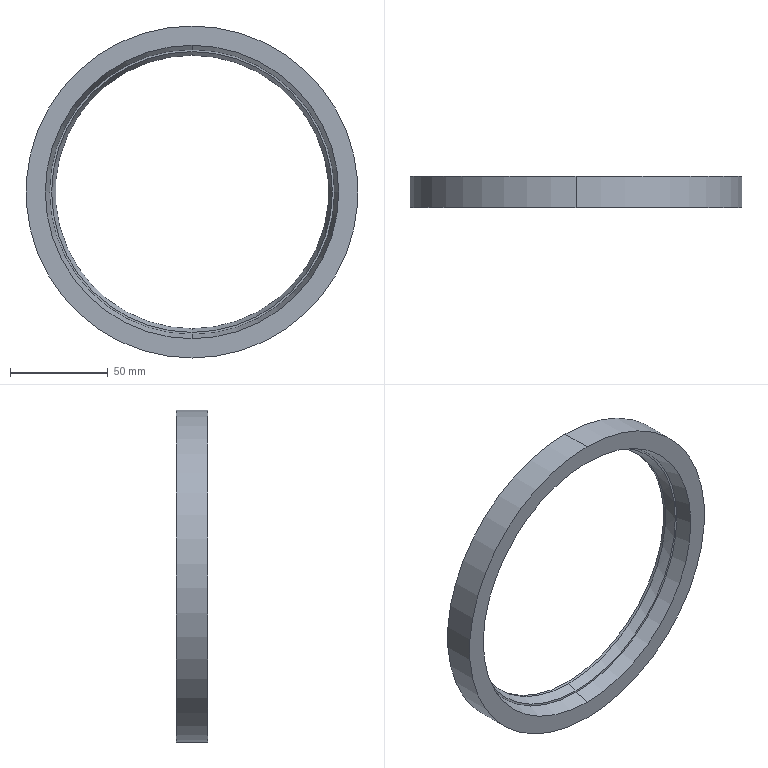Part | STEP file | JB1091-1991 skeleton-type vacuum rubber seal ring 140 | 1 solid | 23 faces | box 170 x 16 x 170 mm | volume 62160 mm3 | cone 8 | cylinder 6 | plane 5 | torus 4 | commonest cylinder face diameters 140 x2 152.823 x2 170 x2
STEP:
#1=CARTESIAN_POINT('',(0.,0.,0.));
#2=DIRECTION('',(0.,0.,1.));
#3=DIRECTION('',(1.,0.,0.));
#4=AXIS2_PLACEMENT_3D('',#1,#2,#3);
#5=CARTESIAN_POINT('',(0.,13.014,76.412));
#6=VERTEX_POINT('',#5);
#7=CARTESIAN_POINT('',(0.,13.014,-76.412));
#8=VERTEX_POINT('',#7);
#9=CARTESIAN_POINT('',(0.,13.014,0.));
#10=DIRECTION('',(0.,1.,0.));
#11=DIRECTION('',(0.,0.,1.));
#12=AXIS2_PLACEMENT_3D('',#9,#10,#11);
#13=CIRCLE('',#12,76.412);
#14=CARTESIAN_POINT('',(0.,10.581,0.));
#15=DIRECTION('',(0.,1.,0.));
#16=DIRECTION('',(0.,0.,1.));
#17=AXIS2_PLACEMENT_3D('',#14,#15,#16);
#18=TOROIDAL_SURFACE('',#17,75.552,2.581);
#19=CARTESIAN_POINT('',(0.,1.231));
#20=DIRECTION('',(1.,0.));
#21=VECTOR('',#20,1.);
#22=LINE('',#19,#21);
#23=(GEOMETRIC_REPRESENTATION_CONTEXT(2)PARAMETRIC_REPRESENTATION_CONTEXT()REPRESENTATION_CONTEXT('',''));
#24=DEFINITIONAL_REPRESENTATION('',(#22),#23);
#25=PCURVE('',#18,#24);
#26=CARTESIAN_POINT('',(0.,0.,0.));
#27=DIRECTION('',(0.,1.,0.));
#28=DIRECTION('',(0.,0.,1.));
#29=AXIS2_PLACEMENT_3D('',#26,#27,#28);
#30=CYLINDRICAL_SURFACE('',#29,76.412);
#31=CARTESIAN_POINT('',(0.,13.014));
#32=DIRECTION('',(1.,0.));
#33=VECTOR('',#32,1.);
#34=LINE('',#31,#33);
#35=(GEOMETRIC_REPRESENTATION_CONTEXT(2)PARAMETRIC_REPRESENTATION_CONTEXT()REPRESENTATION_CONTEXT('',''));
#36=DEFINITIONAL_REPRESENTATION('',(#34),#35);
#37=PCURVE('',#30,#36);
#38=SURFACE_CURVE('',#13,(#25,#37),.PCURVE_S1.);
#39=EDGE_CURVE('',#6,#8,#38,.T.);
#40=ORIENTED_EDGE('',*,*,#39,.T.);
#41=CARTESIAN_POINT('',(0.,10.581,-72.971));
#42=VERTEX_POINT('',#41);
#43=CARTESIAN_POINT('',(0.,10.581,-75.552));
#44=DIRECTION('',(1.,0.,0.));
#45=DIRECTION('',(0.,0.,-1.));
#46=AXIS2_PLACEMENT_3D('',#43,#44,#45);
#47=CIRCLE('',#46,2.581);
#48=CARTESIAN_POINT('',(3.142,0.));
#49=DIRECTION('',(0.,1.));
#50=VECTOR('',#49,1.);
#51=LINE('',#48,#50);
#52=(GEOMETRIC_REPRESENTATION_CONTEXT(2)PARAMETRIC_REPRESENTATION_CONTEXT()REPRESENTATION_CONTEXT('',''));
#53=DEFINITIONAL_REPRESENTATION('',(#51),#52);
#54=PCURVE('',#18,#53);
#55=CARTESIAN_POINT('',(0.,10.581,0.));
#56=DIRECTION('',(0.,1.,0.));
#57=DIRECTION('',(0.,0.,1.));
#58=AXIS2_PLACEMENT_3D('',#55,#56,#57);
#59=TOROIDAL_SURFACE('',#58,75.552,2.581);
#60=CARTESIAN_POINT('',(3.142,0.));
#61=DIRECTION('',(0.,1.));
#62=VECTOR('',#61,1.);
#63=LINE('',#60,#62);
#64=(GEOMETRIC_REPRESENTATION_CONTEXT(2)PARAMETRIC_REPRESENTATION_CONTEXT()REPRESENTATION_CONTEXT('',''));
#65=DEFINITIONAL_REPRESENTATION('',(#63),#64);
#66=PCURVE('',#59,#65);
#67=SURFACE_CURVE('',#47,(#54,#66),.PCURVE_S1.);
#68=EDGE_CURVE('',#8,#42,#67,.T.);
#69=ORIENTED_EDGE('',*,*,#68,.T.);
#70=CARTESIAN_POINT('',(0.,10.581,72.971));
#71=VERTEX_POINT('',#70);
#72=CARTESIAN_POINT('',(0.,10.581,0.));
#73=DIRECTION('',(0.,1.,0.));
#74=DIRECTION('',(0.,0.,1.));
#75=AXIS2_PLACEMENT_3D('',#72,#73,#74);
#76=CIRCLE('',#75,72.971);
#77=CARTESIAN_POINT('',(0.,3.142));
#78=DIRECTION('',(1.,0.));
#79=VECTOR('',#78,1.);
#80=LINE('',#77,#79);
#81=(GEOMETRIC_REPRESENTATION_CONTEXT(2)PARAMETRIC_REPRESENTATION_CONTEXT()REPRESENTATION_CONTEXT('',''));
#82=DEFINITIONAL_REPRESENTATION('',(#80),#81);
#83=PCURVE('',#18,#82);
#84=CARTESIAN_POINT('',(0.,10.581,0.));
#85=DIRECTION('',(0.,1.,0.));
#86=DIRECTION('',(0.,0.,1.));
#87=AXIS2_PLACEMENT_3D('',#84,#85,#86);
#88=TOROIDAL_SURFACE('',#87,75.552,2.581);
#89=CARTESIAN_POINT('',(0.,3.142));
#90=DIRECTION('',(1.,0.));
#91=VECTOR('',#90,1.);
#92=LINE('',#89,#91);
#93=(GEOMETRIC_REPRESENTATION_CONTEXT(2)PARAMETRIC_REPRESENTATION_CONTEXT()REPRESENTATION_CONTEXT('',''));
#94=DEFINITIONAL_REPRESENTATION('',(#92),#93);
#95=PCURVE('',#88,#94);
#96=SURFACE_CURVE('',#76,(#83,#95),.PCURVE_S1.);
#97=EDGE_CURVE('',#71,#42,#96,.T.);
#98=ORIENTED_EDGE('',*,*,#97,.F.);
#99=CARTESIAN_POINT('',(0.,10.581,75.552));
#100=DIRECTION('',(-1.,0.,0.));
#101=DIRECTION('',(0.,0.,1.));
#102=AXIS2_PLACEMENT_3D('',#99,#100,#101);
#103=CIRCLE('',#102,2.581);
#104=CARTESIAN_POINT('',(0.,0.));
#105=DIRECTION('',(0.,1.));
#106=VECTOR('',#105,1.);
#107=LINE('',#104,#106);
#108=(GEOMETRIC_REPRESENTATION_CONTEXT(2)PARAMETRIC_REPRESENTATION_CONTEXT()REPRESENTATION_CONTEXT('',''));
#109=DEFINITIONAL_REPRESENTATION('',(#107),#108);
#110=PCURVE('',#18,#109);
#111=CARTESIAN_POINT('',(6.283,0.));
#112=DIRECTION('',(0.,1.));
#113=VECTOR('',#112,1.);
#114=LINE('',#111,#113);
#115=(GEOMETRIC_REPRESENTATION_CONTEXT(2)PARAMETRIC_REPRESENTATION_CONTEXT()REPRESENTATION_CONTEXT('',''));
#116=DEFINITIONAL_REPRESENTATION('',(#114),#115);
#117=PCURVE('',#59,#116);
#118=SURFACE_CURVE('',#103,(#110,#117),.PCURVE_S1.);
#119=EDGE_CURVE('',#6,#71,#118,.T.);
#120=ORIENTED_EDGE('',*,*,#119,.F.);
#121=EDGE_LOOP('',(#40,#69,#98,#120));
#122=FACE_BOUND('',#121,.F.);
#123=ADVANCED_FACE('',(#122),#18,.F.);
#124=CARTESIAN_POINT('',(0.,13.014,0.));
#125=DIRECTION('',(0.,1.,0.));
#126=DIRECTION('',(0.,0.,1.));
#127=AXIS2_PLACEMENT_3D('',#124,#125,#126);
#128=CIRCLE('',#127,76.412);
#129=CARTESIAN_POINT('',(0.,1.231));
#130=DIRECTION('',(1.,0.));
#131=VECTOR('',#130,1.);
#132=LINE('',#129,#131);
#133=(GEOMETRIC_REPRESENTATION_CONTEXT(2)PARAMETRIC_REPRESENTATION_CONTEXT()REPRESENTATION_CONTEXT('',''));
#134=DEFINITIONAL_REPRESENTATION('',(#132),#133);
#135=PCURVE('',#59,#134);
#136=CARTESIAN_POINT('',(0.,0.,0.));
#137=DIRECTION('',(0.,1.,0.));
#138=DIRECTION('',(0.,0.,1.));
#139=AXIS2_PLACEMENT_3D('',#136,#137,#138);
#140=CYLINDRICAL_SURFACE('',#139,76.412);
#141=CARTESIAN_POINT('',(0.,13.014));
#142=DIRECTION('',(1.,0.));
#143=VECTOR('',#142,1.);
#144=LINE('',#141,#143);
#145=(GEOMETRIC_REPRESENTATION_CONTEXT(2)PARAMETRIC_REPRESENTATION_CONTEXT()REPRESENTATION_CONTEXT('',''));
#146=DEFINITIONAL_REPRESENTATION('',(#144),#145);
#147=PCURVE('',#140,#146);
#148=SURFACE_CURVE('',#128,(#135,#147),.PCURVE_S1.);
#149=EDGE_CURVE('',#8,#6,#148,.T.);
#150=ORIENTED_EDGE('',*,*,#149,.T.);
#151=ORIENTED_EDGE('',*,*,#119,.T.);
#152=CARTESIAN_POINT('',(0.,10.581,0.));
#153=DIRECTION('',(0.,1.,0.));
#154=DIRECTION('',(0.,0.,1.));
#155=AXIS2_PLACEMENT_3D('',#152,#153,#154);
#156=CIRCLE('',#155,72.971);
#157=CARTESIAN_POINT('',(0.,3.142));
#158=DIRECTION('',(1.,0.));
#159=VECTOR('',#158,1.);
#160=LINE('',#157,#159);
#161=(GEOMETRIC_REPRESENTATION_CONTEXT(2)PARAMETRIC_REPRESENTATION_CONTEXT()REPRESENTATION_CONTEXT('',''));
#162=DEFINITIONAL_REPRESENTATION('',(#160),#161);
#163=PCURVE('',#59,#162);
#164=CARTESIAN_POINT('',(0.,10.581,0.));
#165=DIRECTION('',(0.,1.,0.));
#166=DIRECTION('',(0.,0.,1.));
#167=AXIS2_PLACEMENT_3D('',#164,#165,#166);
#168=TOROIDAL_SURFACE('',#167,75.552,2.581);
#169=CARTESIAN_POINT('',(0.,3.142));
#170=DIRECTION('',(1.,0.));
#171=VECTOR('',#170,1.);
#172=LINE('',#169,#171);
#173=(GEOMETRIC_REPRESENTATION_CONTEXT(2)PARAMETRIC_REPRESENTATION_CONTEXT()REPRESENTATION_CONTEXT('',''));
#174=DEFINITIONAL_REPRESENTATION('',(#172),#173);
#175=PCURVE('',#168,#174);
#176=SURFACE_CURVE('',#156,(#163,#175),.PCURVE_S1.);
#177=EDGE_CURVE('',#42,#71,#176,.T.);
#178=ORIENTED_EDGE('',*,*,#177,.F.);
#179=ORIENTED_EDGE('',*,*,#68,.F.);
#180=EDGE_LOOP('',(#150,#151,#178,#179));
#181=FACE_BOUND('',#180,.F.);
#182=ADVANCED_FACE('',(#181),#59,.F.);
#183=CARTESIAN_POINT('',(0.,0.,85.));
#184=VERTEX_POINT('',#183);
#185=CARTESIAN_POINT('',(0.,0.,-85.));
#186=VERTEX_POINT('',#185);
#187=CARTESIAN_POINT('',(0.,0.,0.));
#188=DIRECTION('',(0.,1.,0.));
#189=DIRECTION('',(0.,0.,1.));
#190=AXIS2_PLACEMENT_3D('',#187,#188,#189);
#191=CIRCLE('',#190,85.);
#192=CARTESIAN_POINT('',(0.,0.,0.));
#193=DIRECTION('',(0.,1.,0.));
#194=DIRECTION('',(0.,0.,1.));
#195=AXIS2_PLACEMENT_3D('',#192,#193,#194);
#196=CYLINDRICAL_SURFACE('',#195,85.);
#197=CARTESIAN_POINT('',(0.,0.));
#198=DIRECTION('',(1.,0.));
#199=VECTOR('',#198,1.);
#200=LINE('',#197,#199);
#201=(GEOMETRIC_REPRESENTATION_CONTEXT(2)PARAMETRIC_REPRESENTATION_CONTEXT()REPRESENTATION_CONTEXT('',''));
#202=DEFINITIONAL_REPRESENTATION('',(#200),#201);
#203=PCURVE('',#196,#202);
#204=CARTESIAN_POINT('',(-85.,0.,0.));
#205=DIRECTION('',(0.,-1.,0.));
#206=DIRECTION('',(0.,0.,-1.));
#207=AXIS2_PLACEMENT_3D('',#204,#205,#206);
#208=PLANE('',#207);
#209=CARTESIAN_POINT('',(-85.,85.));
#210=CARTESIAN_POINT('',(-85.,232.224));
#211=CARTESIAN_POINT('',(42.5,158.612));
#212=CARTESIAN_POINT('',(170.,85.));
#213=CARTESIAN_POINT('',(42.5,11.388));
#214=CARTESIAN_POINT('',(-85.,-62.224));
#215=CARTESIAN_POINT('',(-85.,85.));
#216=(BOUNDED_CURVE()B_SPLINE_CURVE(2,(#209,#210,#211,#212,#213,#214,#215),.UNSPECIFIED.,.T.,.F.)B_SPLINE_CURVE_WITH_KNOTS((1,2,2,2,2,1),(-2.094,0.,2.094,4.189,6.283,8.378),.UNSPECIFIED.)CURVE()GEOMETRIC_REPRESENTATION_ITEM()RATIONAL_B_SPLINE_CURVE((1.,0.5,1.,0.5,1.,0.5,1.))REPRESENTATION_ITEM(''));
#217=(GEOMETRIC_REPRESENTATION_CONTEXT(2)PARAMETRIC_REPRESENTATION_CONTEXT()REPRESENTATION_CONTEXT('',''));
#218=DEFINITIONAL_REPRESENTATION('',(#216),#217);
#219=PCURVE('',#208,#218);
#220=SURFACE_CURVE('',#191,(#203,#219),.PCURVE_S1.);
#221=EDGE_CURVE('',#184,#186,#220,.T.);
#222=ORIENTED_EDGE('',*,*,#221,.T.);
#223=CARTESIAN_POINT('',(0.,16.,-85.));
#224=VERTEX_POINT('',#223);
#225=CARTESIAN_POINT('',(0.,0.,-85.));
#226=DIRECTION('',(0.,1.,0.));
#227=VECTOR('',#226,1.);
#228=LINE('',#225,#227);
#229=CARTESIAN_POINT('',(3.142,0.));
#230=DIRECTION('',(0.,1.));
#231=VECTOR('',#230,1.);
#232=LINE('',#229,#231);
#233=(GEOMETRIC_REPRESENTATION_CONTEXT(2)PARAMETRIC_REPRESENTATION_CONTEXT()REPRESENTATION_CONTEXT('',''));
#234=DEFINITIONAL_REPRESENTATION('',(#232),#233);
#235=PCURVE('',#196,#234);
#236=CARTESIAN_POINT('',(0.,0.,0.));
#237=DIRECTION('',(0.,1.,0.));
#238=DIRECTION('',(0.,0.,1.));
#239=AXIS2_PLACEMENT_3D('',#236,#237,#238);
#240=CYLINDRICAL_SURFACE('',#239,85.);
#241=CARTESIAN_POINT('',(3.142,0.));
#242=DIRECTION('',(0.,1.));
#243=VECTOR('',#242,1.);
#244=LINE('',#241,#243);
#245=(GEOMETRIC_REPRESENTATION_CONTEXT(2)PARAMETRIC_REPRESENTATION_CONTEXT()REPRESENTATION_CONTEXT('',''));
#246=DEFINITIONAL_REPRESENTATION('',(#244),#245);
#247=PCURVE('',#240,#246);
#248=SURFACE_CURVE('',#228,(#235,#247),.PCURVE_S1.);
#249=EDGE_CURVE('',#186,#224,#248,.T.);
#250=ORIENTED_EDGE('',*,*,#249,.T.);
#251=CARTESIAN_POINT('',(0.,16.,85.));
#252=VERTEX_POINT('',#251);
#253=CARTESIAN_POINT('',(0.,16.,0.));
#254=DIRECTION('',(0.,1.,0.));
#255=DIRECTION('',(0.,0.,1.));
#256=AXIS2_PLACEMENT_3D('',#253,#254,#255);
#257=CIRCLE('',#256,85.);
#258=CARTESIAN_POINT('',(0.,16.));
#259=DIRECTION('',(1.,0.));
#260=VECTOR('',#259,1.);
#261=LINE('',#258,#260);
#262=(GEOMETRIC_REPRESENTATION_CONTEXT(2)PARAMETRIC_REPRESENTATION_CONTEXT()REPRESENTATION_CONTEXT('',''));
#263=DEFINITIONAL_REPRESENTATION('',(#261),#262);
#264=PCURVE('',#196,#263);
#265=CARTESIAN_POINT('',(-82.419,16.,0.));
#266=DIRECTION('',(0.,1.,0.));
#267=DIRECTION('',(0.,0.,1.));
#268=AXIS2_PLACEMENT_3D('',#265,#266,#267);
#269=PLANE('',#268);
#270=CARTESIAN_POINT('',(0.,82.419));
#271=DIRECTION('',(1.,0.));
#272=AXIS2_PLACEMENT_2D('',#270,#271);
#273=CIRCLE('',#272,85.);
#274=(GEOMETRIC_REPRESENTATION_CONTEXT(2)PARAMETRIC_REPRESENTATION_CONTEXT()REPRESENTATION_CONTEXT('',''));
#275=DEFINITIONAL_REPRESENTATION('',(#273),#274);
#276=PCURVE('',#269,#275);
#277=SURFACE_CURVE('',#257,(#264,#276),.PCURVE_S1.);
#278=EDGE_CURVE('',#252,#224,#277,.T.);
#279=ORIENTED_EDGE('',*,*,#278,.F.);
#280=CARTESIAN_POINT('',(0.,0.,85.));
#281=DIRECTION('',(0.,1.,0.));
#282=VECTOR('',#281,1.);
#283=LINE('',#280,#282);
#284=CARTESIAN_POINT('',(0.,0.));
#285=DIRECTION('',(0.,1.));
#286=VECTOR('',#285,1.);
#287=LINE('',#284,#286);
#288=(GEOMETRIC_REPRESENTATION_CONTEXT(2)PARAMETRIC_REPRESENTATION_CONTEXT()REPRESENTATION_CONTEXT('',''));
#289=DEFINITIONAL_REPRESENTATION('',(#287),#288);
#290=PCURVE('',#196,#289);
#291=CARTESIAN_POINT('',(6.283,0.));
#292=DIRECTION('',(0.,1.));
#293=VECTOR('',#292,1.);
#294=LINE('',#291,#293);
#295=(GEOMETRIC_REPRESENTATION_CONTEXT(2)PARAMETRIC_REPRESENTATION_CONTEXT()REPRESENTATION_CONTEXT('',''));
#296=DEFINITIONAL_REPRESENTATION('',(#294),#295);
#297=PCURVE('',#240,#296);
#298=SURFACE_CURVE('',#283,(#290,#297),.PCURVE_S1.);
#299=EDGE_CURVE('',#184,#252,#298,.T.);
#300=ORIENTED_EDGE('',*,*,#299,.F.);
#301=EDGE_LOOP('',(#222,#250,#279,#300));
#302=FACE_BOUND('',#301,.T.);
#303=ADVANCED_FACE('',(#302),#196,.T.);
#304=CARTESIAN_POINT('',(0.,8.,-72.971));
#305=VERTEX_POINT('',#304);
#306=CARTESIAN_POINT('',(0.,0.,-75.114));
#307=VERTEX_POINT('',#306);
#308=CARTESIAN_POINT('',(0.,0.,-75.114));
#309=DIRECTION('',(0.,-0.9659,-0.2588));
#310=VECTOR('',#309,1.);
#311=LINE('',#308,#310);
#312=CARTESIAN_POINT('',(0.,0.,0.));
#313=DIRECTION('',(0.,-1.,0.));
#314=DIRECTION('',(0.,0.,-1.));
#315=AXIS2_PLACEMENT_3D('',#312,#313,#314);
#316=CONICAL_SURFACE('',#315,75.114,0.2618);
#317=CARTESIAN_POINT('',(6.283,0.));
#318=DIRECTION('',(0.,1.));
#319=VECTOR('',#318,1.);
#320=LINE('',#317,#319);
#321=(GEOMETRIC_REPRESENTATION_CONTEXT(2)PARAMETRIC_REPRESENTATION_CONTEXT()REPRESENTATION_CONTEXT('',''));
#322=DEFINITIONAL_REPRESENTATION('',(#320),#321);
#323=PCURVE('',#316,#322);
#324=CARTESIAN_POINT('',(0.,0.,0.));
#325=DIRECTION('',(0.,-1.,0.));
#326=DIRECTION('',(0.,0.,-1.));
#327=AXIS2_PLACEMENT_3D('',#324,#325,#326);
#328=CONICAL_SURFACE('',#327,75.114,0.2618);
#329=CARTESIAN_POINT('',(0.,0.));
#330=DIRECTION('',(0.,1.));
#331=VECTOR('',#330,1.);
#332=LINE('',#329,#331);
#333=(GEOMETRIC_REPRESENTATION_CONTEXT(2)PARAMETRIC_REPRESENTATION_CONTEXT()REPRESENTATION_CONTEXT('',''));
#334=DEFINITIONAL_REPRESENTATION('',(#332),#333);
#335=PCURVE('',#328,#334);
#336=SURFACE_CURVE('',#311,(#323,#335),.PCURVE_S1.);
#337=EDGE_CURVE('',#305,#307,#336,.T.);
#338=ORIENTED_EDGE('',*,*,#337,.T.);
#339=CARTESIAN_POINT('',(0.,0.,75.114));
#340=VERTEX_POINT('',#339);
#341=CARTESIAN_POINT('',(0.,0.,0.));
#342=DIRECTION('',(0.,1.,0.));
#343=DIRECTION('',(0.,0.,1.));
#344=AXIS2_PLACEMENT_3D('',#341,#342,#343);
#345=CIRCLE('',#344,75.114);
#346=CARTESIAN_POINT('',(9.425,0.));
#347=DIRECTION('',(-1.,0.));
#348=VECTOR('',#347,1.);
#349=LINE('',#346,#348);
#350=(GEOMETRIC_REPRESENTATION_CONTEXT(2)PARAMETRIC_REPRESENTATION_CONTEXT()REPRESENTATION_CONTEXT('',''));
#351=DEFINITIONAL_REPRESENTATION('',(#349),#350);
#352=PCURVE('',#316,#351);
#353=CARTESIAN_POINT('',(-75.114,85.));
#354=CARTESIAN_POINT('',(-75.114,215.102));
#355=CARTESIAN_POINT('',(37.557,150.051));
#356=CARTESIAN_POINT('',(150.229,85.));
#357=CARTESIAN_POINT('',(37.557,19.949));
#358=CARTESIAN_POINT('',(-75.114,-45.102));
#359=CARTESIAN_POINT('',(-75.114,85.));
#360=(BOUNDED_CURVE()B_SPLINE_CURVE(2,(#353,#354,#355,#356,#357,#358,#359),.UNSPECIFIED.,.T.,.F.)B_SPLINE_CURVE_WITH_KNOTS((1,2,2,2,2,1),(-2.094,0.,2.094,4.189,6.283,8.378),.UNSPECIFIED.)CURVE()GEOMETRIC_REPRESENTATION_ITEM()RATIONAL_B_SPLINE_CURVE((1.,0.5,1.,0.5,1.,0.5,1.))REPRESENTATION_ITEM(''));
#361=(GEOMETRIC_REPRESENTATION_CONTEXT(2)PARAMETRIC_REPRESENTATION_CONTEXT()REPRESENTATION_CONTEXT('',''));
#362=DEFINITIONAL_REPRESENTATION('',(#360),#361);
#363=PCURVE('',#208,#362);
#364=SURFACE_CURVE('',#345,(#352,#363),.PCURVE_S1.);
#365=EDGE_CURVE('',#307,#340,#364,.T.);
#366=ORIENTED_EDGE('',*,*,#365,.T.);
#367=CARTESIAN_POINT('',(0.,8.,72.971));
#368=VERTEX_POINT('',#367);
#369=CARTESIAN_POINT('',(0.,0.,75.114));
#370=DIRECTION('',(0.,-0.9659,0.2588));
#371=VECTOR('',#370,1.);
#372=LINE('',#369,#371);
#373=CARTESIAN_POINT('',(3.142,0.));
#374=DIRECTION('',(0.,1.));
#375=VECTOR('',#374,1.);
#376=LINE('',#373,#375);
#377=(GEOMETRIC_REPRESENTATION_CONTEXT(2)PARAMETRIC_REPRESENTATION_CONTEXT()REPRESENTATION_CONTEXT('',''));
#378=DEFINITIONAL_REPRESENTATION('',(#376),#377);
#379=PCURVE('',#316,#378);
#380=CARTESIAN_POINT('',(3.142,0.));
#381=DIRECTION('',(0.,1.));
#382=VECTOR('',#381,1.);
#383=LINE('',#380,#382);
#384=(GEOMETRIC_REPRESENTATION_CONTEXT(2)PARAMETRIC_REPRESENTATION_CONTEXT()REPRESENTATION_CONTEXT('',''));
#385=DEFINITIONAL_REPRESENTATION('',(#383),#384);
#386=PCURVE('',#328,#385);
#387=SURFACE_CURVE('',#372,(#379,#386),.PCURVE_S1.);
#388=EDGE_CURVE('',#368,#340,#387,.T.);
#389=ORIENTED_EDGE('',*,*,#388,.F.);
#390=CARTESIAN_POINT('',(0.,8.,0.));
#391=DIRECTION('',(0.,1.,0.));
#392=DIRECTION('',(0.,0.,1.));
#393=AXIS2_PLACEMENT_3D('',#390,#391,#392);
#394=CIRCLE('',#393,72.971);
#395=CARTESIAN_POINT('',(9.425,-8.));
#396=DIRECTION('',(-1.,0.));
#397=VECTOR('',#396,1.);
#398=LINE('',#395,#397);
#399=(GEOMETRIC_REPRESENTATION_CONTEXT(2)PARAMETRIC_REPRESENTATION_CONTEXT()REPRESENTATION_CONTEXT('',''));
#400=DEFINITIONAL_REPRESENTATION('',(#398),#399);
#401=PCURVE('',#316,#400);
#402=CARTESIAN_POINT('',(-72.971,8.,0.));
#403=DIRECTION('',(0.,-1.,0.));
#404=DIRECTION('',(0.,0.,-1.));
#405=AXIS2_PLACEMENT_3D('',#402,#403,#404);
#406=PLANE('',#405);
#407=CARTESIAN_POINT('',(-72.971,72.971));
#408=CARTESIAN_POINT('',(-72.971,199.36));
#409=CARTESIAN_POINT('',(36.485,136.166));
#410=CARTESIAN_POINT('',(145.942,72.971));
#411=CARTESIAN_POINT('',(36.485,9.776));
#412=CARTESIAN_POINT('',(-72.971,-53.418));
#413=CARTESIAN_POINT('',(-72.971,72.971));
#414=(BOUNDED_CURVE()B_SPLINE_CURVE(2,(#407,#408,#409,#410,#411,#412,#413),.UNSPECIFIED.,.T.,.F.)B_SPLINE_CURVE_WITH_KNOTS((1,2,2,2,2,1),(-2.094,0.,2.094,4.189,6.283,8.378),.UNSPECIFIED.)CURVE()GEOMETRIC_REPRESENTATION_ITEM()RATIONAL_B_SPLINE_CURVE((1.,0.5,1.,0.5,1.,0.5,1.))REPRESENTATION_ITEM(''));
#415=(GEOMETRIC_REPRESENTATION_CONTEXT(2)PARAMETRIC_REPRESENTATION_CONTEXT()REPRESENTATION_CONTEXT('',''));
#416=DEFINITIONAL_REPRESENTATION('',(#414),#415);
#417=PCURVE('',#406,#416);
#418=SURFACE_CURVE('',#394,(#401,#417),.PCURVE_S1.);
#419=EDGE_CURVE('',#305,#368,#418,.T.);
#420=ORIENTED_EDGE('',*,*,#419,.F.);
#421=EDGE_LOOP('',(#338,#366,#389,#420));
#422=FACE_BOUND('',#421,.F.);
#423=ADVANCED_FACE('',(#422),#316,.F.);
#424=CARTESIAN_POINT('',(0.,13.161,-70.));
#425=VERTEX_POINT('',#424);
#426=CARTESIAN_POINT('',(0.,8.,-71.879));
#427=VERTEX_POINT('',#426);
#428=CARTESIAN_POINT('',(0.,8.,-71.879));
#429=DIRECTION('',(0.,-0.9397,-0.342));
#430=VECTOR('',#429,1.);
#431=LINE('',#428,#430);
#432=CARTESIAN_POINT('',(0.,8.,0.));
#433=DIRECTION('',(0.,-1.,0.));
#434=DIRECTION('',(0.,0.,-1.));
#435=AXIS2_PLACEMENT_3D('',#432,#433,#434);
#436=CONICAL_SURFACE('',#435,71.879,0.3491);
#437=CARTESIAN_POINT('',(6.283,0.));
#438=DIRECTION('',(0.,1.));
#439=VECTOR('',#438,1.);
#440=LINE('',#437,#439);
#441=(GEOMETRIC_REPRESENTATION_CONTEXT(2)PARAMETRIC_REPRESENTATION_CONTEXT()REPRESENTATION_CONTEXT('',''));
#442=DEFINITIONAL_REPRESENTATION('',(#440),#441);
#443=PCURVE('',#436,#442);
#444=CARTESIAN_POINT('',(0.,8.,0.));
#445=DIRECTION('',(0.,-1.,0.));
#446=DIRECTION('',(0.,0.,-1.));
#447=AXIS2_PLACEMENT_3D('',#444,#445,#446);
#448=CONICAL_SURFACE('',#447,71.879,0.3491);
#449=CARTESIAN_POINT('',(0.,0.));
#450=DIRECTION('',(0.,1.));
#451=VECTOR('',#450,1.);
#452=LINE('',#449,#451);
#453=(GEOMETRIC_REPRESENTATION_CONTEXT(2)PARAMETRIC_REPRESENTATION_CONTEXT()REPRESENTATION_CONTEXT('',''));
#454=DEFINITIONAL_REPRESENTATION('',(#452),#453);
#455=PCURVE('',#448,#454);
#456=SURFACE_CURVE('',#431,(#443,#455),.PCURVE_S1.);
#457=EDGE_CURVE('',#425,#427,#456,.T.);
#458=ORIENTED_EDGE('',*,*,#457,.T.);
#459=CARTESIAN_POINT('',(0.,8.,71.879));
#460=VERTEX_POINT('',#459);
#461=CARTESIAN_POINT('',(0.,8.,0.));
#462=DIRECTION('',(0.,1.,0.));
#463=DIRECTION('',(0.,0.,1.));
#464=AXIS2_PLACEMENT_3D('',#461,#462,#463);
#465=CIRCLE('',#464,71.879);
#466=CARTESIAN_POINT('',(9.425,0.));
#467=DIRECTION('',(-1.,0.));
#468=VECTOR('',#467,1.);
#469=LINE('',#466,#468);
#470=(GEOMETRIC_REPRESENTATION_CONTEXT(2)PARAMETRIC_REPRESENTATION_CONTEXT()REPRESENTATION_CONTEXT('',''));
#471=DEFINITIONAL_REPRESENTATION('',(#469),#470);
#472=PCURVE('',#436,#471);
#473=CARTESIAN_POINT('',(-71.879,72.971));
#474=CARTESIAN_POINT('',(-71.879,197.468));
#475=CARTESIAN_POINT('',(35.939,135.22));
#476=CARTESIAN_POINT('',(143.757,72.971));
#477=CARTESIAN_POINT('',(35.939,10.722));
#478=CARTESIAN_POINT('',(-71.879,-51.526));
#479=CARTESIAN_POINT('',(-71.879,72.971));
#480=(BOUNDED_CURVE()B_SPLINE_CURVE(2,(#473,#474,#475,#476,#477,#478,#479),.UNSPECIFIED.,.T.,.F.)B_SPLINE_CURVE_WITH_KNOTS((1,2,2,2,2,1),(-2.094,0.,2.094,4.189,6.283,8.378),.UNSPECIFIED.)CURVE()GEOMETRIC_REPRESENTATION_ITEM()RATIONAL_B_SPLINE_CURVE((1.,0.5,1.,0.5,1.,0.5,1.))REPRESENTATION_ITEM(''));
#481=(GEOMETRIC_REPRESENTATION_CONTEXT(2)PARAMETRIC_REPRESENTATION_CONTEXT()REPRESENTATION_CONTEXT('',''));
#482=DEFINITIONAL_REPRESENTATION('',(#480),#481);
#483=PCURVE('',#406,#482);
#484=SURFACE_CURVE('',#465,(#472,#483),.PCURVE_S1.);
#485=EDGE_CURVE('',#427,#460,#484,.T.);
#486=ORIENTED_EDGE('',*,*,#485,.T.);
#487=CARTESIAN_POINT('',(0.,13.161,70.));
#488=VERTEX_POINT('',#487);
#489=CARTESIAN_POINT('',(0.,8.,71.879));
#490=DIRECTION('',(0.,-0.9397,0.342));
#491=VECTOR('',#490,1.);
#492=LINE('',#489,#491);
#493=CARTESIAN_POINT('',(3.142,0.));
#494=DIRECTION('',(0.,1.));
#495=VECTOR('',#494,1.);
#496=LINE('',#493,#495);
#497=(GEOMETRIC_REPRESENTATION_CONTEXT(2)PARAMETRIC_REPRESENTATION_CONTEXT()REPRESENTATION_CONTEXT('',''));
#498=DEFINITIONAL_REPRESENTATION('',(#496),#497);
#499=PCURVE('',#436,#498);
#500=CARTESIAN_POINT('',(3.142,0.));
#501=DIRECTION('',(0.,1.));
#502=VECTOR('',#501,1.);
#503=LINE('',#500,#502);
#504=(GEOMETRIC_REPRESENTATION_CONTEXT(2)PARAMETRIC_REPRESENTATION_CONTEXT()REPRESENTATION_CONTEXT('',''));
#505=DEFINITIONAL_REPRESENTATION('',(#503),#504);
#506=PCURVE('',#448,#505);
#507=SURFACE_CURVE('',#492,(#499,#506),.PCURVE_S1.);
#508=EDGE_CURVE('',#488,#460,#507,.T.);
#509=ORIENTED_EDGE('',*,*,#508,.F.);
#510=CARTESIAN_POINT('',(0.,13.161,0.));
#511=DIRECTION('',(0.,1.,0.));
#512=DIRECTION('',(0.,0.,1.));
#513=AXIS2_PLACEMENT_3D('',#510,#511,#512);
#514=CIRCLE('',#513,70.);
#515=CARTESIAN_POINT('',(9.425,-5.161));
#516=DIRECTION('',(-1.,0.));
#517=VECTOR('',#516,1.);
#518=LINE('',#515,#517);
#519=(GEOMETRIC_REPRESENTATION_CONTEXT(2)PARAMETRIC_REPRESENTATION_CONTEXT()REPRESENTATION_CONTEXT('',''));
#520=DEFINITIONAL_REPRESENTATION('',(#518),#519);
#521=PCURVE('',#436,#520);
#522=CARTESIAN_POINT('',(0.,0.,0.));
#523=DIRECTION('',(0.,1.,0.));
#524=DIRECTION('',(0.,0.,1.));
#525=AXIS2_PLACEMENT_3D('',#522,#523,#524);
#526=CYLINDRICAL_SURFACE('',#525,70.);
#527=CARTESIAN_POINT('',(0.,13.161));
#528=DIRECTION('',(1.,0.));
#529=VECTOR('',#528,1.);
#530=LINE('',#527,#529);
#531=(GEOMETRIC_REPRESENTATION_CONTEXT(2)PARAMETRIC_REPRESENTATION_CONTEXT()REPRESENTATION_CONTEXT('',''));
#532=DEFINITIONAL_REPRESENTATION('',(#530),#531);
#533=PCURVE('',#526,#532);
#534=SURFACE_CURVE('',#514,(#521,#533),.PCURVE_S1.);
#535=EDGE_CURVE('',#425,#488,#534,.T.);
#536=ORIENTED_EDGE('',*,*,#535,.F.);
#537=EDGE_LOOP('',(#458,#486,#509,#536));
#538=FACE_BOUND('',#537,.F.);
#539=ADVANCED_FACE('',(#538),#436,.F.);
#540=CARTESIAN_POINT('',(0.,14.581,70.));
#541=VERTEX_POINT('',#540);
#542=CARTESIAN_POINT('',(0.,0.,70.));
#543=DIRECTION('',(0.,1.,0.));
#544=VECTOR('',#543,1.);
#545=LINE('',#542,#544);
#546=CARTESIAN_POINT('',(6.283,0.));
#547=DIRECTION('',(0.,1.));
#548=VECTOR('',#547,1.);
#549=LINE('',#546,#548);
#550=(GEOMETRIC_REPRESENTATION_CONTEXT(2)PARAMETRIC_REPRESENTATION_CONTEXT()REPRESENTATION_CONTEXT('',''));
#551=DEFINITIONAL_REPRESENTATION('',(#549),#550);
#552=PCURVE('',#526,#551);
#553=CARTESIAN_POINT('',(0.,0.,0.));
#554=DIRECTION('',(0.,1.,0.));
#555=DIRECTION('',(0.,0.,1.));
#556=AXIS2_PLACEMENT_3D('',#553,#554,#555);
#557=CYLINDRICAL_SURFACE('',#556,70.);
#558=CARTESIAN_POINT('',(0.,0.));
#559=DIRECTION('',(0.,1.));
#560=VECTOR('',#559,1.);
#561=LINE('',#558,#560);
#562=(GEOMETRIC_REPRESENTATION_CONTEXT(2)PARAMETRIC_REPRESENTATION_CONTEXT()REPRESENTATION_CONTEXT('',''));
#563=DEFINITIONAL_REPRESENTATION('',(#561),#562);
#564=PCURVE('',#557,#563);
#565=SURFACE_CURVE('',#545,(#552,#564),.PCURVE_S1.);
#566=EDGE_CURVE('',#488,#541,#565,.T.);
#567=ORIENTED_EDGE('',*,*,#566,.T.);
#568=CARTESIAN_POINT('',(0.,14.581,-70.));
#569=VERTEX_POINT('',#568);
#570=CARTESIAN_POINT('',(0.,14.581,0.));
#571=DIRECTION('',(0.,1.,0.));
#572=DIRECTION('',(0.,0.,1.));
#573=AXIS2_PLACEMENT_3D('',#570,#571,#572);
#574=CIRCLE('',#573,70.);
#575=CARTESIAN_POINT('',(0.,14.581));
#576=DIRECTION('',(1.,0.));
#577=VECTOR('',#576,1.);
#578=LINE('',#575,#577);
#579=(GEOMETRIC_REPRESENTATION_CONTEXT(2)PARAMETRIC_REPRESENTATION_CONTEXT()REPRESENTATION_CONTEXT('',''));
#580=DEFINITIONAL_REPRESENTATION('',(#578),#579);
#581=PCURVE('',#526,#580);
#582=CARTESIAN_POINT('',(-70.,14.581,0.));
#583=DIRECTION('',(0.,1.,0.));
#584=DIRECTION('',(0.,0.,1.));
#585=AXIS2_PLACEMENT_3D('',#582,#583,#584);
#586=PLANE('',#585);
#587=CARTESIAN_POINT('',(0.,70.));
#588=DIRECTION('',(1.,0.));
#589=AXIS2_PLACEMENT_2D('',#587,#588);
#590=CIRCLE('',#589,70.);
#591=(GEOMETRIC_REPRESENTATION_CONTEXT(2)PARAMETRIC_REPRESENTATION_CONTEXT()REPRESENTATION_CONTEXT('',''));
#592=DEFINITIONAL_REPRESENTATION('',(#590),#591);
#593=PCURVE('',#586,#592);
#594=SURFACE_CURVE('',#574,(#581,#593),.PCURVE_S1.);
#595=EDGE_CURVE('',#569,#541,#594,.T.);
#596=ORIENTED_EDGE('',*,*,#595,.F.);
#597=CARTESIAN_POINT('',(0.,0.,-70.));
#598=DIRECTION('',(0.,1.,0.));
#599=VECTOR('',#598,1.);
#600=LINE('',#597,#599);
#601=CARTESIAN_POINT('',(3.142,0.));
#602=DIRECTION('',(0.,1.));
#603=VECTOR('',#602,1.);
#604=LINE('',#601,#603);
#605=(GEOMETRIC_REPRESENTATION_CONTEXT(2)PARAMETRIC_REPRESENTATION_CONTEXT()REPRESENTATION_CONTEXT('',''));
#606=DEFINITIONAL_REPRESENTATION('',(#604),#605);
#607=PCURVE('',#526,#606);
#608=CARTESIAN_POINT('',(3.142,0.));
#609=DIRECTION('',(0.,1.));
#610=VECTOR('',#609,1.);
#611=LINE('',#608,#610);
#612=(GEOMETRIC_REPRESENTATION_CONTEXT(2)PARAMETRIC_REPRESENTATION_CONTEXT()REPRESENTATION_CONTEXT('',''));
#613=DEFINITIONAL_REPRESENTATION('',(#611),#612);
#614=PCURVE('',#557,#613);
#615=SURFACE_CURVE('',#600,(#607,#614),.PCURVE_S1.);
#616=EDGE_CURVE('',#425,#569,#615,.T.);
#617=ORIENTED_EDGE('',*,*,#616,.F.);
#618=ORIENTED_EDGE('',*,*,#535,.T.);
#619=EDGE_LOOP('',(#567,#596,#617,#618));
#620=FACE_BOUND('',#619,.F.);
#621=ADVANCED_FACE('',(#620),#526,.F.);
#622=ORIENTED_EDGE('',*,*,#39,.T.);
#623=CARTESIAN_POINT('',(0.,14.581,-76.412));
#624=VERTEX_POINT('',#623);
#625=CARTESIAN_POINT('',(0.,0.,-76.412));
#626=DIRECTION('',(0.,1.,0.));
#627=VECTOR('',#626,1.);
#628=LINE('',#625,#627);
#629=CARTESIAN_POINT('',(3.142,0.));
#630=DIRECTION('',(0.,1.));
#631=VECTOR('',#630,1.);
#632=LINE('',#629,#631);
#633=(GEOMETRIC_REPRESENTATION_CONTEXT(2)PARAMETRIC_REPRESENTATION_CONTEXT()REPRESENTATION_CONTEXT('',''));
#634=DEFINITIONAL_REPRESENTATION('',(#632),#633);
#635=PCURVE('',#30,#634);
#636=CARTESIAN_POINT('',(3.142,0.));
#637=DIRECTION('',(0.,1.));
#638=VECTOR('',#637,1.);
#639=LINE('',#636,#638);
#640=(GEOMETRIC_REPRESENTATION_CONTEXT(2)PARAMETRIC_REPRESENTATION_CONTEXT()REPRESENTATION_CONTEXT('',''));
#641=DEFINITIONAL_REPRESENTATION('',(#639),#640);
#642=PCURVE('',#140,#641);
#643=SURFACE_CURVE('',#628,(#635,#642),.PCURVE_S1.);
#644=EDGE_CURVE('',#8,#624,#643,.T.);
#645=ORIENTED_EDGE('',*,*,#644,.T.);
#646=CARTESIAN_POINT('',(0.,14.581,76.412));
#647=VERTEX_POINT('',#646);
#648=CARTESIAN_POINT('',(0.,14.581,0.));
#649=DIRECTION('',(0.,1.,0.));
#650=DIRECTION('',(0.,0.,1.));
#651=AXIS2_PLACEMENT_3D('',#648,#649,#650);
#652=CIRCLE('',#651,76.412);
#653=CARTESIAN_POINT('',(0.,14.581));
#654=DIRECTION('',(1.,0.));
#655=VECTOR('',#654,1.);
#656=LINE('',#653,#655);
#657=(GEOMETRIC_REPRESENTATION_CONTEXT(2)PARAMETRIC_REPRESENTATION_CONTEXT()REPRESENTATION_CONTEXT('',''));
#658=DEFINITIONAL_REPRESENTATION('',(#656),#657);
#659=PCURVE('',#30,#658);
#660=CARTESIAN_POINT('',(0.,70.));
#661=DIRECTION('',(1.,0.));
#662=AXIS2_PLACEMENT_2D('',#660,#661);
#663=CIRCLE('',#662,76.412);
#664=(GEOMETRIC_REPRESENTATION_CONTEXT(2)PARAMETRIC_REPRESENTATION_CONTEXT()REPRESENTATION_CONTEXT('',''));
#665=DEFINITIONAL_REPRESENTATION('',(#663),#664);
#666=PCURVE('',#586,#665);
#667=SURFACE_CURVE('',#652,(#659,#666),.PCURVE_S1.);
#668=EDGE_CURVE('',#647,#624,#667,.T.);
#669=ORIENTED_EDGE('',*,*,#668,.F.);
#670=CARTESIAN_POINT('',(0.,0.,76.412));
#671=DIRECTION('',(0.,1.,0.));
#672=VECTOR('',#671,1.);
#673=LINE('',#670,#672);
#674=CARTESIAN_POINT('',(0.,0.));
#675=DIRECTION('',(0.,1.));
#676=VECTOR('',#675,1.);
#677=LINE('',#674,#676);
#678=(GEOMETRIC_REPRESENTATION_CONTEXT(2)PARAMETRIC_REPRESENTATION_CONTEXT()REPRESENTATION_CONTEXT('',''));
#679=DEFINITIONAL_REPRESENTATION('',(#677),#678);
#680=PCURVE('',#30,#679);
#681=CARTESIAN_POINT('',(6.283,0.));
#682=DIRECTION('',(0.,1.));
#683=VECTOR('',#682,1.);
#684=LINE('',#681,#683);
#685=(GEOMETRIC_REPRESENTATION_CONTEXT(2)PARAMETRIC_REPRESENTATION_CONTEXT()REPRESENTATION_CONTEXT('',''));
#686=DEFINITIONAL_REPRESENTATION('',(#684),#685);
#687=PCURVE('',#140,#686);
#688=SURFACE_CURVE('',#673,(#680,#687),.PCURVE_S1.);
#689=EDGE_CURVE('',#6,#647,#688,.T.);
#690=ORIENTED_EDGE('',*,*,#689,.F.);
#691=EDGE_LOOP('',(#622,#645,#669,#690));
#692=FACE_BOUND('',#691,.T.);
#693=ADVANCED_FACE('',(#692),#30,.T.);
#694=CARTESIAN_POINT('',(0.,8.,75.552));
#695=VERTEX_POINT('',#694);
#696=CARTESIAN_POINT('',(0.,10.581,75.552));
#697=DIRECTION('',(-1.,0.,0.));
#698=DIRECTION('',(0.,0.,1.));
#699=AXIS2_PLACEMENT_3D('',#696,#697,#698);
#700=CIRCLE('',#699,2.581);
#701=CARTESIAN_POINT('',(6.283,0.));
#702=DIRECTION('',(0.,1.));
#703=VECTOR('',#702,1.);
#704=LINE('',#701,#703);
#705=(GEOMETRIC_REPRESENTATION_CONTEXT(2)PARAMETRIC_REPRESENTATION_CONTEXT()REPRESENTATION_CONTEXT('',''));
#706=DEFINITIONAL_REPRESENTATION('',(#704),#705);
#707=PCURVE('',#168,#706);
#708=CARTESIAN_POINT('',(0.,0.));
#709=DIRECTION('',(0.,1.));
#710=VECTOR('',#709,1.);
#711=LINE('',#708,#710);
#712=(GEOMETRIC_REPRESENTATION_CONTEXT(2)PARAMETRIC_REPRESENTATION_CONTEXT()REPRESENTATION_CONTEXT('',''));
#713=DEFINITIONAL_REPRESENTATION('',(#711),#712);
#714=PCURVE('',#88,#713);
#715=SURFACE_CURVE('',#700,(#707,#714),.PCURVE_S1.);
#716=EDGE_CURVE('',#71,#695,#715,.T.);
#717=ORIENTED_EDGE('',*,*,#716,.T.);
#718=CARTESIAN_POINT('',(0.,8.,-75.552));
#719=VERTEX_POINT('',#718);
#720=CARTESIAN_POINT('',(0.,8.,0.));
#721=DIRECTION('',(0.,1.,0.));
#722=DIRECTION('',(0.,0.,1.));
#723=AXIS2_PLACEMENT_3D('',#720,#721,#722);
#724=CIRCLE('',#723,75.552);
#725=CARTESIAN_POINT('',(0.,4.712));
#726=DIRECTION('',(1.,0.));
#727=VECTOR('',#726,1.);
#728=LINE('',#725,#727);
#729=(GEOMETRIC_REPRESENTATION_CONTEXT(2)PARAMETRIC_REPRESENTATION_CONTEXT()REPRESENTATION_CONTEXT('',''));
#730=DEFINITIONAL_REPRESENTATION('',(#728),#729);
#731=PCURVE('',#168,#730);
#732=CARTESIAN_POINT('',(0.,8.,0.));
#733=DIRECTION('',(0.,-1.,0.));
#734=DIRECTION('',(0.,0.,-1.));
#735=AXIS2_PLACEMENT_3D('',#732,#733,#734);
#736=CONICAL_SURFACE('',#735,75.552,0.2618);
#737=CARTESIAN_POINT('',(9.425,0.));
#738=DIRECTION('',(-1.,0.));
#739=VECTOR('',#738,1.);
#740=LINE('',#737,#739);
#741=(GEOMETRIC_REPRESENTATION_CONTEXT(2)PARAMETRIC_REPRESENTATION_CONTEXT()REPRESENTATION_CONTEXT('',''));
#742=DEFINITIONAL_REPRESENTATION('',(#740),#741);
#743=PCURVE('',#736,#742);
#744=SURFACE_CURVE('',#724,(#731,#743),.PCURVE_S1.);
#745=EDGE_CURVE('',#719,#695,#744,.T.);
#746=ORIENTED_EDGE('',*,*,#745,.F.);
#747=CARTESIAN_POINT('',(0.,10.581,-75.552));
#748=DIRECTION('',(1.,0.,0.));
#749=DIRECTION('',(0.,0.,-1.));
#750=AXIS2_PLACEMENT_3D('',#747,#748,#749);
#751=CIRCLE('',#750,2.581);
#752=CARTESIAN_POINT('',(3.142,0.));
#753=DIRECTION('',(0.,1.));
#754=VECTOR('',#753,1.);
#755=LINE('',#752,#754);
#756=(GEOMETRIC_REPRESENTATION_CONTEXT(2)PARAMETRIC_REPRESENTATION_CONTEXT()REPRESENTATION_CONTEXT('',''));
#757=DEFINITIONAL_REPRESENTATION('',(#755),#756);
#758=PCURVE('',#168,#757);
#759=CARTESIAN_POINT('',(3.142,0.));
#760=DIRECTION('',(0.,1.));
#761=VECTOR('',#760,1.);
#762=LINE('',#759,#761);
#763=(GEOMETRIC_REPRESENTATION_CONTEXT(2)PARAMETRIC_REPRESENTATION_CONTEXT()REPRESENTATION_CONTEXT('',''));
#764=DEFINITIONAL_REPRESENTATION('',(#762),#763);
#765=PCURVE('',#88,#764);
#766=SURFACE_CURVE('',#751,(#758,#765),.PCURVE_S1.);
#767=EDGE_CURVE('',#42,#719,#766,.T.);
#768=ORIENTED_EDGE('',*,*,#767,.F.);
#769=ORIENTED_EDGE('',*,*,#177,.T.);
#770=EDGE_LOOP('',(#717,#746,#768,#769));
#771=FACE_BOUND('',#770,.F.);
#772=ADVANCED_FACE('',(#771),#168,.F.);
#773=CARTESIAN_POINT('',(0.,8.,0.));
#774=DIRECTION('',(0.,1.,0.));
#775=DIRECTION('',(0.,0.,1.));
#776=AXIS2_PLACEMENT_3D('',#773,#774,#775);
#777=CIRCLE('',#776,75.552);
#778=CARTESIAN_POINT('',(0.,8.,0.));
#779=DIRECTION('',(0.,-1.,0.));
#780=DIRECTION('',(0.,0.,-1.));
#781=AXIS2_PLACEMENT_3D('',#778,#779,#780);
#782=CONICAL_SURFACE('',#781,75.552,0.2618);
#783=CARTESIAN_POINT('',(3.142,0.));
#784=DIRECTION('',(-1.,0.));
#785=VECTOR('',#784,1.);
#786=LINE('',#783,#785);
#787=(GEOMETRIC_REPRESENTATION_CONTEXT(2)PARAMETRIC_REPRESENTATION_CONTEXT()REPRESENTATION_CONTEXT('',''));
#788=DEFINITIONAL_REPRESENTATION('',(#786),#787);
#789=PCURVE('',#782,#788);
#790=CARTESIAN_POINT('',(0.,4.712));
#791=DIRECTION('',(1.,0.));
#792=VECTOR('',#791,1.);
#793=LINE('',#790,#792);
#794=(GEOMETRIC_REPRESENTATION_CONTEXT(2)PARAMETRIC_REPRESENTATION_CONTEXT()REPRESENTATION_CONTEXT('',''));
#795=DEFINITIONAL_REPRESENTATION('',(#793),#794);
#796=PCURVE('',#88,#795);
#797=SURFACE_CURVE('',#777,(#789,#796),.PCURVE_S1.);
#798=EDGE_CURVE('',#695,#719,#797,.T.);
#799=ORIENTED_EDGE('',*,*,#798,.F.);
#800=CARTESIAN_POINT('',(0.,4.,76.623));
#801=VERTEX_POINT('',#800);
#802=CARTESIAN_POINT('',(0.,8.,75.552));
#803=DIRECTION('',(0.,-0.9659,0.2588));
#804=VECTOR('',#803,1.);
#805=LINE('',#802,#804);
#806=CARTESIAN_POINT('',(3.142,0.));
#807=DIRECTION('',(0.,1.));
#808=VECTOR('',#807,1.);
#809=LINE('',#806,#808);
#810=(GEOMETRIC_REPRESENTATION_CONTEXT(2)PARAMETRIC_REPRESENTATION_CONTEXT()REPRESENTATION_CONTEXT('',''));
#811=DEFINITIONAL_REPRESENTATION('',(#809),#810);
#812=PCURVE('',#782,#811);
#813=CARTESIAN_POINT('',(3.142,0.));
#814=DIRECTION('',(0.,1.));
#815=VECTOR('',#814,1.);
#816=LINE('',#813,#815);
#817=(GEOMETRIC_REPRESENTATION_CONTEXT(2)PARAMETRIC_REPRESENTATION_CONTEXT()REPRESENTATION_CONTEXT('',''));
#818=DEFINITIONAL_REPRESENTATION('',(#816),#817);
#819=PCURVE('',#736,#818);
#820=SURFACE_CURVE('',#805,(#812,#819),.PCURVE_S1.);
#821=EDGE_CURVE('',#695,#801,#820,.T.);
#822=ORIENTED_EDGE('',*,*,#821,.T.);
#823=CARTESIAN_POINT('',(0.,4.,-76.623));
#824=VERTEX_POINT('',#823);
#825=CARTESIAN_POINT('',(0.,4.,0.));
#826=DIRECTION('',(0.,1.,0.));
#827=DIRECTION('',(0.,0.,1.));
#828=AXIS2_PLACEMENT_3D('',#825,#826,#827);
#829=CIRCLE('',#828,76.623);
#830=CARTESIAN_POINT('',(3.142,4.));
#831=DIRECTION('',(-1.,0.));
#832=VECTOR('',#831,1.);
#833=LINE('',#830,#832);
#834=(GEOMETRIC_REPRESENTATION_CONTEXT(2)PARAMETRIC_REPRESENTATION_CONTEXT()REPRESENTATION_CONTEXT('',''));
#835=DEFINITIONAL_REPRESENTATION('',(#833),#834);
#836=PCURVE('',#782,#835);
#837=CARTESIAN_POINT('',(-76.623,4.,0.));
#838=DIRECTION('',(0.,1.,0.));
#839=DIRECTION('',(0.,0.,1.));
#840=AXIS2_PLACEMENT_3D('',#837,#838,#839);
#841=PLANE('',#840);
#842=CARTESIAN_POINT('',(0.,76.623));
#843=DIRECTION('',(1.,0.));
#844=AXIS2_PLACEMENT_2D('',#842,#843);
#845=CIRCLE('',#844,76.623);
#846=(GEOMETRIC_REPRESENTATION_CONTEXT(2)PARAMETRIC_REPRESENTATION_CONTEXT()REPRESENTATION_CONTEXT('',''));
#847=DEFINITIONAL_REPRESENTATION('',(#845),#846);
#848=PCURVE('',#841,#847);
#849=SURFACE_CURVE('',#829,(#836,#848),.PCURVE_S1.);
#850=EDGE_CURVE('',#801,#824,#849,.T.);
#851=ORIENTED_EDGE('',*,*,#850,.T.);
#852=CARTESIAN_POINT('',(0.,8.,-75.552));
#853=DIRECTION('',(0.,-0.9659,-0.2588));
#854=VECTOR('',#853,1.);
#855=LINE('',#852,#854);
#856=CARTESIAN_POINT('',(0.,0.));
#857=DIRECTION('',(0.,1.));
#858=VECTOR('',#857,1.);
#859=LINE('',#856,#858);
#860=(GEOMETRIC_REPRESENTATION_CONTEXT(2)PARAMETRIC_REPRESENTATION_CONTEXT()REPRESENTATION_CONTEXT('',''));
#861=DEFINITIONAL_REPRESENTATION('',(#859),#860);
#862=PCURVE('',#782,#861);
#863=CARTESIAN_POINT('',(6.283,0.));
#864=DIRECTION('',(0.,1.));
#865=VECTOR('',#864,1.);
#866=LINE('',#863,#865);
#867=(GEOMETRIC_REPRESENTATION_CONTEXT(2)PARAMETRIC_REPRESENTATION_CONTEXT()REPRESENTATION_CONTEXT('',''));
#868=DEFINITIONAL_REPRESENTATION('',(#866),#867);
#869=PCURVE('',#736,#868);
#870=SURFACE_CURVE('',#855,(#862,#869),.PCURVE_S1.);
#871=EDGE_CURVE('',#719,#824,#870,.T.);
#872=ORIENTED_EDGE('',*,*,#871,.F.);
#873=EDGE_LOOP('',(#799,#822,#851,#872));
#874=FACE_BOUND('',#873,.T.);
#875=ADVANCED_FACE('',(#874),#782,.T.);
#876=CARTESIAN_POINT('',(0.,4.,79.204));
#877=VERTEX_POINT('',#876);
#878=CARTESIAN_POINT('',(0.,16.,82.419));
#879=VERTEX_POINT('',#878);
#880=CARTESIAN_POINT('',(0.,4.,79.204));
#881=DIRECTION('',(0.,0.9659,0.2588));
#882=VECTOR('',#881,1.);
#883=LINE('',#880,#882);
#884=CARTESIAN_POINT('',(0.,4.,0.));
#885=DIRECTION('',(0.,1.,0.));
#886=DIRECTION('',(0.,0.,1.));
#887=AXIS2_PLACEMENT_3D('',#884,#885,#886);
#888=CONICAL_SURFACE('',#887,79.204,0.2618);
#889=CARTESIAN_POINT('',(6.283,0.));
#890=DIRECTION('',(0.,1.));
#891=VECTOR('',#890,1.);
#892=LINE('',#889,#891);
#893=(GEOMETRIC_REPRESENTATION_CONTEXT(2)PARAMETRIC_REPRESENTATION_CONTEXT()REPRESENTATION_CONTEXT('',''));
#894=DEFINITIONAL_REPRESENTATION('',(#892),#893);
#895=PCURVE('',#888,#894);
#896=CARTESIAN_POINT('',(0.,4.,0.));
#897=DIRECTION('',(0.,1.,0.));
#898=DIRECTION('',(0.,0.,1.));
#899=AXIS2_PLACEMENT_3D('',#896,#897,#898);
#900=CONICAL_SURFACE('',#899,79.204,0.2618);
#901=CARTESIAN_POINT('',(0.,0.));
#902=DIRECTION('',(0.,1.));
#903=VECTOR('',#902,1.);
#904=LINE('',#901,#903);
#905=(GEOMETRIC_REPRESENTATION_CONTEXT(2)PARAMETRIC_REPRESENTATION_CONTEXT()REPRESENTATION_CONTEXT('',''));
#906=DEFINITIONAL_REPRESENTATION('',(#904),#905);
#907=PCURVE('',#900,#906);
#908=SURFACE_CURVE('',#883,(#895,#907),.PCURVE_S1.);
#909=EDGE_CURVE('',#877,#879,#908,.T.);
#910=ORIENTED_EDGE('',*,*,#909,.T.);
#911=CARTESIAN_POINT('',(0.,16.,-82.419));
#912=VERTEX_POINT('',#911);
#913=CARTESIAN_POINT('',(0.,16.,0.));
#914=DIRECTION('',(0.,1.,0.));
#915=DIRECTION('',(0.,0.,1.));
#916=AXIS2_PLACEMENT_3D('',#913,#914,#915);
#917=CIRCLE('',#916,82.419);
#918=CARTESIAN_POINT('',(0.,12.));
#919=DIRECTION('',(1.,0.));
#920=VECTOR('',#919,1.);
#921=LINE('',#918,#920);
#922=(GEOMETRIC_REPRESENTATION_CONTEXT(2)PARAMETRIC_REPRESENTATION_CONTEXT()REPRESENTATION_CONTEXT('',''));
#923=DEFINITIONAL_REPRESENTATION('',(#921),#922);
#924=PCURVE('',#888,#923);
#925=CARTESIAN_POINT('',(0.,82.419));
#926=DIRECTION('',(1.,0.));
#927=AXIS2_PLACEMENT_2D('',#925,#926);
#928=CIRCLE('',#927,82.419);
#929=(GEOMETRIC_REPRESENTATION_CONTEXT(2)PARAMETRIC_REPRESENTATION_CONTEXT()REPRESENTATION_CONTEXT('',''));
#930=DEFINITIONAL_REPRESENTATION('',(#928),#929);
#931=PCURVE('',#269,#930);
#932=SURFACE_CURVE('',#917,(#924,#931),.PCURVE_S1.);
#933=EDGE_CURVE('',#912,#879,#932,.T.);
#934=ORIENTED_EDGE('',*,*,#933,.F.);
#935=CARTESIAN_POINT('',(0.,4.,-79.204));
#936=VERTEX_POINT('',#935);
#937=CARTESIAN_POINT('',(0.,4.,-79.204));
#938=DIRECTION('',(0.,0.9659,-0.2588));
#939=VECTOR('',#938,1.);
#940=LINE('',#937,#939);
#941=CARTESIAN_POINT('',(3.142,0.));
#942=DIRECTION('',(0.,1.));
#943=VECTOR('',#942,1.);
#944=LINE('',#941,#943);
#945=(GEOMETRIC_REPRESENTATION_CONTEXT(2)PARAMETRIC_REPRESENTATION_CONTEXT()REPRESENTATION_CONTEXT('',''));
#946=DEFINITIONAL_REPRESENTATION('',(#944),#945);
#947=PCURVE('',#888,#946);
#948=CARTESIAN_POINT('',(3.142,0.));
#949=DIRECTION('',(0.,1.));
#950=VECTOR('',#949,1.);
#951=LINE('',#948,#950);
#952=(GEOMETRIC_REPRESENTATION_CONTEXT(2)PARAMETRIC_REPRESENTATION_CONTEXT()REPRESENTATION_CONTEXT('',''));
#953=DEFINITIONAL_REPRESENTATION('',(#951),#952);
#954=PCURVE('',#900,#953);
#955=SURFACE_CURVE('',#940,(#947,#954),.PCURVE_S1.);
#956=EDGE_CURVE('',#936,#912,#955,.T.);
#957=ORIENTED_EDGE('',*,*,#956,.F.);
#958=CARTESIAN_POINT('',(0.,4.,0.));
#959=DIRECTION('',(0.,1.,0.));
#960=DIRECTION('',(0.,0.,1.));
#961=AXIS2_PLACEMENT_3D('',#958,#959,#960);
#962=CIRCLE('',#961,79.204);
#963=CARTESIAN_POINT('',(0.,0.));
#964=DIRECTION('',(1.,0.));
#965=VECTOR('',#964,1.);
#966=LINE('',#963,#965);
#967=(GEOMETRIC_REPRESENTATION_CONTEXT(2)PARAMETRIC_REPRESENTATION_CONTEXT()REPRESENTATION_CONTEXT('',''));
#968=DEFINITIONAL_REPRESENTATION('',(#966),#967);
#969=PCURVE('',#888,#968);
#970=CARTESIAN_POINT('',(0.,76.623));
#971=DIRECTION('',(1.,0.));
#972=AXIS2_PLACEMENT_2D('',#970,#971);
#973=CIRCLE('',#972,79.204);
#974=(GEOMETRIC_REPRESENTATION_CONTEXT(2)PARAMETRIC_REPRESENTATION_CONTEXT()REPRESENTATION_CONTEXT('',''));
#975=DEFINITIONAL_REPRESENTATION('',(#973),#974);
#976=PCURVE('',#841,#975);
#977=SURFACE_CURVE('',#962,(#969,#976),.PCURVE_S1.);
#978=EDGE_CURVE('',#936,#877,#977,.T.);
#979=ORIENTED_EDGE('',*,*,#978,.T.);
#980=EDGE_LOOP('',(#910,#934,#957,#979));
#981=FACE_BOUND('',#980,.F.);
#982=ADVANCED_FACE('',(#981),#888,.F.);
#983=ORIENTED_EDGE('',*,*,#278,.T.);
#984=CARTESIAN_POINT('',(0.,16.,0.));
#985=DIRECTION('',(0.,1.,0.));
#986=DIRECTION('',(0.,0.,1.));
#987=AXIS2_PLACEMENT_3D('',#984,#985,#986);
#988=CIRCLE('',#987,85.);
#989=CARTESIAN_POINT('',(0.,82.419));
#990=DIRECTION('',(1.,0.));
#991=AXIS2_PLACEMENT_2D('',#989,#990);
#992=CIRCLE('',#991,85.);
#993=(GEOMETRIC_REPRESENTATION_CONTEXT(2)PARAMETRIC_REPRESENTATION_CONTEXT()REPRESENTATION_CONTEXT('',''));
#994=DEFINITIONAL_REPRESENTATION('',(#992),#993);
#995=PCURVE('',#269,#994);
#996=CARTESIAN_POINT('',(0.,16.));
#997=DIRECTION('',(1.,0.));
#998=VECTOR('',#997,1.);
#999=LINE('',#996,#998);
#1000=(GEOMETRIC_REPRESENTATION_CONTEXT(2)PARAMETRIC_REPRESENTATION_CONTEXT()REPRESENTATION_CONTEXT('',''));
#1001=DEFINITIONAL_REPRESENTATION('',(#999),#1000);
#1002=PCURVE('',#240,#1001);
#1003=SURFACE_CURVE('',#988,(#995,#1002),.PCURVE_S1.);
#1004=EDGE_CURVE('',#224,#252,#1003,.T.);
#1005=ORIENTED_EDGE('',*,*,#1004,.T.);
#1006=EDGE_LOOP('',(#983,#1005));
#1007=FACE_BOUND('',#1006,.T.);
#1008=CARTESIAN_POINT('',(0.,16.,0.));
#1009=DIRECTION('',(0.,1.,0.));
#1010=DIRECTION('',(0.,0.,1.));
#1011=AXIS2_PLACEMENT_3D('',#1008,#1009,#1010);
#1012=CIRCLE('',#1011,82.419);
#1013=CARTESIAN_POINT('',(0.,82.419));
#1014=DIRECTION('',(1.,0.));
#1015=AXIS2_PLACEMENT_2D('',#1013,#1014);
#1016=CIRCLE('',#1015,82.419);
#1017=(GEOMETRIC_REPRESENTATION_CONTEXT(2)PARAMETRIC_REPRESENTATION_CONTEXT()REPRESENTATION_CONTEXT('',''));
#1018=DEFINITIONAL_REPRESENTATION('',(#1016),#1017);
#1019=PCURVE('',#269,#1018);
#1020=CARTESIAN_POINT('',(0.,12.));
#1021=DIRECTION('',(1.,0.));
#1022=VECTOR('',#1021,1.);
#1023=LINE('',#1020,#1022);
#1024=(GEOMETRIC_REPRESENTATION_CONTEXT(2)PARAMETRIC_REPRESENTATION_CONTEXT()REPRESENTATION_CONTEXT('',''));
#1025=DEFINITIONAL_REPRESENTATION('',(#1023),#1024);
#1026=PCURVE('',#900,#1025);
#1027=SURFACE_CURVE('',#1012,(#1019,#1026),.PCURVE_S1.);
#1028=EDGE_CURVE('',#879,#912,#1027,.T.);
#1029=ORIENTED_EDGE('',*,*,#1028,.F.);
#1030=ORIENTED_EDGE('',*,*,#933,.F.);
#1031=EDGE_LOOP('',(#1029,#1030));
#1032=FACE_BOUND('',#1031,.T.);
#1033=ADVANCED_FACE('',(#1007,#1032),#269,.T.);
#1034=ORIENTED_EDGE('',*,*,#1028,.F.);
#1035=ORIENTED_EDGE('',*,*,#909,.F.);
#1036=CARTESIAN_POINT('',(0.,4.,0.));
#1037=DIRECTION('',(0.,1.,0.));
#1038=DIRECTION('',(0.,0.,1.));
#1039=AXIS2_PLACEMENT_3D('',#1036,#1037,#1038);
#1040=CIRCLE('',#1039,79.204);
#1041=CARTESIAN_POINT('',(0.,0.));
#1042=DIRECTION('',(1.,0.));
#1043=VECTOR('',#1042,1.);
#1044=LINE('',#1041,#1043);
#1045=(GEOMETRIC_REPRESENTATION_CONTEXT(2)PARAMETRIC_REPRESENTATION_CONTEXT()REPRESENTATION_CONTEXT('',''));
#1046=DEFINITIONAL_REPRESENTATION('',(#1044),#1045);
#1047=PCURVE('',#900,#1046);
#1048=CARTESIAN_POINT('',(0.,76.623));
#1049=DIRECTION('',(1.,0.));
#1050=AXIS2_PLACEMENT_2D('',#1048,#1049);
#1051=CIRCLE('',#1050,79.204);
#1052=(GEOMETRIC_REPRESENTATION_CONTEXT(2)PARAMETRIC_REPRESENTATION_CONTEXT()REPRESENTATION_CONTEXT('',''));
#1053=DEFINITIONAL_REPRESENTATION('',(#1051),#1052);
#1054=PCURVE('',#841,#1053);
#1055=SURFACE_CURVE('',#1040,(#1047,#1054),.PCURVE_S1.);
#1056=EDGE_CURVE('',#877,#936,#1055,.T.);
#1057=ORIENTED_EDGE('',*,*,#1056,.T.);
#1058=ORIENTED_EDGE('',*,*,#956,.T.);
#1059=EDGE_LOOP('',(#1034,#1035,#1057,#1058));
#1060=FACE_BOUND('',#1059,.F.);
#1061=ADVANCED_FACE('',(#1060),#900,.F.);
#1062=ORIENTED_EDGE('',*,*,#1056,.T.);
#1063=ORIENTED_EDGE('',*,*,#978,.T.);
#1064=EDGE_LOOP('',(#1062,#1063));
#1065=FACE_BOUND('',#1064,.T.);
#1066=CARTESIAN_POINT('',(0.,4.,0.));
#1067=DIRECTION('',(0.,1.,0.));
#1068=DIRECTION('',(0.,0.,1.));
#1069=AXIS2_PLACEMENT_3D('',#1066,#1067,#1068);
#1070=CIRCLE('',#1069,76.623);
#1071=CARTESIAN_POINT('',(0.,76.623));
#1072=DIRECTION('',(1.,0.));
#1073=AXIS2_PLACEMENT_2D('',#1071,#1072);
#1074=CIRCLE('',#1073,76.623);
#1075=(GEOMETRIC_REPRESENTATION_CONTEXT(2)PARAMETRIC_REPRESENTATION_CONTEXT()REPRESENTATION_CONTEXT('',''));
#1076=DEFINITIONAL_REPRESENTATION('',(#1074),#1075);
#1077=PCURVE('',#841,#1076);
#1078=CARTESIAN_POINT('',(9.425,4.));
#1079=DIRECTION('',(-1.,0.));
#1080=VECTOR('',#1079,1.);
#1081=LINE('',#1078,#1080);
#1082=(GEOMETRIC_REPRESENTATION_CONTEXT(2)PARAMETRIC_REPRESENTATION_CONTEXT()REPRESENTATION_CONTEXT('',''));
#1083=DEFINITIONAL_REPRESENTATION('',(#1081),#1082);
#1084=PCURVE('',#736,#1083);
#1085=SURFACE_CURVE('',#1070,(#1077,#1084),.PCURVE_S1.);
#1086=EDGE_CURVE('',#824,#801,#1085,.T.);
#1087=ORIENTED_EDGE('',*,*,#1086,.F.);
#1088=ORIENTED_EDGE('',*,*,#850,.F.);
#1089=EDGE_LOOP('',(#1087,#1088));
#1090=FACE_BOUND('',#1089,.T.);
#1091=ADVANCED_FACE('',(#1065,#1090),#841,.T.);
#1092=ORIENTED_EDGE('',*,*,#821,.F.);
#1093=ORIENTED_EDGE('',*,*,#745,.F.);
#1094=ORIENTED_EDGE('',*,*,#871,.T.);
#1095=ORIENTED_EDGE('',*,*,#1086,.T.);
#1096=EDGE_LOOP('',(#1092,#1093,#1094,#1095));
#1097=FACE_BOUND('',#1096,.T.);
#1098=ADVANCED_FACE('',(#1097),#736,.T.);
#1099=ORIENTED_EDGE('',*,*,#767,.T.);
#1100=ORIENTED_EDGE('',*,*,#798,.F.);
#1101=ORIENTED_EDGE('',*,*,#716,.F.);
#1102=ORIENTED_EDGE('',*,*,#97,.T.);
#1103=EDGE_LOOP('',(#1099,#1100,#1101,#1102));
#1104=FACE_BOUND('',#1103,.F.);
#1105=ADVANCED_FACE('',(#1104),#88,.F.);
#1106=ORIENTED_EDGE('',*,*,#644,.F.);
#1107=ORIENTED_EDGE('',*,*,#149,.T.);
#1108=ORIENTED_EDGE('',*,*,#689,.T.);
#1109=CARTESIAN_POINT('',(0.,14.581,0.));
#1110=DIRECTION('',(0.,1.,0.));
#1111=DIRECTION('',(0.,0.,1.));
#1112=AXIS2_PLACEMENT_3D('',#1109,#1110,#1111);
#1113=CIRCLE('',#1112,76.412);
#1114=CARTESIAN_POINT('',(0.,14.581));
#1115=DIRECTION('',(1.,0.));
#1116=VECTOR('',#1115,1.);
#1117=LINE('',#1114,#1116);
#1118=(GEOMETRIC_REPRESENTATION_CONTEXT(2)PARAMETRIC_REPRESENTATION_CONTEXT()REPRESENTATION_CONTEXT('',''));
#1119=DEFINITIONAL_REPRESENTATION('',(#1117),#1118);
#1120=PCURVE('',#140,#1119);
#1121=CARTESIAN_POINT('',(0.,70.));
#1122=DIRECTION('',(1.,0.));
#1123=AXIS2_PLACEMENT_2D('',#1121,#1122);
#1124=CIRCLE('',#1123,76.412);
#1125=(GEOMETRIC_REPRESENTATION_CONTEXT(2)PARAMETRIC_REPRESENTATION_CONTEXT()REPRESENTATION_CONTEXT('',''));
#1126=DEFINITIONAL_REPRESENTATION('',(#1124),#1125);
#1127=PCURVE('',#586,#1126);
#1128=SURFACE_CURVE('',#1113,(#1120,#1127),.PCURVE_S1.);
#1129=EDGE_CURVE('',#624,#647,#1128,.T.);
#1130=ORIENTED_EDGE('',*,*,#1129,.F.);
#1131=EDGE_LOOP('',(#1106,#1107,#1108,#1130));
#1132=FACE_BOUND('',#1131,.T.);
#1133=ADVANCED_FACE('',(#1132),#140,.T.);
#1134=ORIENTED_EDGE('',*,*,#668,.T.);
#1135=ORIENTED_EDGE('',*,*,#1129,.T.);
#1136=EDGE_LOOP('',(#1134,#1135));
#1137=FACE_BOUND('',#1136,.T.);
#1138=CARTESIAN_POINT('',(0.,14.581,0.));
#1139=DIRECTION('',(0.,1.,0.));
#1140=DIRECTION('',(0.,0.,1.));
#1141=AXIS2_PLACEMENT_3D('',#1138,#1139,#1140);
#1142=CIRCLE('',#1141,70.);
#1143=CARTESIAN_POINT('',(0.,70.));
#1144=DIRECTION('',(1.,0.));
#1145=AXIS2_PLACEMENT_2D('',#1143,#1144);
#1146=CIRCLE('',#1145,70.);
#1147=(GEOMETRIC_REPRESENTATION_CONTEXT(2)PARAMETRIC_REPRESENTATION_CONTEXT()REPRESENTATION_CONTEXT('',''));
#1148=DEFINITIONAL_REPRESENTATION('',(#1146),#1147);
#1149=PCURVE('',#586,#1148);
#1150=CARTESIAN_POINT('',(0.,14.581));
#1151=DIRECTION('',(1.,0.));
#1152=VECTOR('',#1151,1.);
#1153=LINE('',#1150,#1152);
#1154=(GEOMETRIC_REPRESENTATION_CONTEXT(2)PARAMETRIC_REPRESENTATION_CONTEXT()REPRESENTATION_CONTEXT('',''));
#1155=DEFINITIONAL_REPRESENTATION('',(#1153),#1154);
#1156=PCURVE('',#557,#1155);
#1157=SURFACE_CURVE('',#1142,(#1149,#1156),.PCURVE_S1.);
#1158=EDGE_CURVE('',#541,#569,#1157,.T.);
#1159=ORIENTED_EDGE('',*,*,#1158,.F.);
#1160=ORIENTED_EDGE('',*,*,#595,.F.);
#1161=EDGE_LOOP('',(#1159,#1160));
#1162=FACE_BOUND('',#1161,.T.);
#1163=ADVANCED_FACE('',(#1137,#1162),#586,.T.);
#1164=ORIENTED_EDGE('',*,*,#1158,.F.);
#1165=ORIENTED_EDGE('',*,*,#566,.F.);
#1166=CARTESIAN_POINT('',(0.,13.161,0.));
#1167=DIRECTION('',(0.,1.,0.));
#1168=DIRECTION('',(0.,0.,1.));
#1169=AXIS2_PLACEMENT_3D('',#1166,#1167,#1168);
#1170=CIRCLE('',#1169,70.);
#1171=CARTESIAN_POINT('',(0.,13.161));
#1172=DIRECTION('',(1.,0.));
#1173=VECTOR('',#1172,1.);
#1174=LINE('',#1171,#1173);
#1175=(GEOMETRIC_REPRESENTATION_CONTEXT(2)PARAMETRIC_REPRESENTATION_CONTEXT()REPRESENTATION_CONTEXT('',''));
#1176=DEFINITIONAL_REPRESENTATION('',(#1174),#1175);
#1177=PCURVE('',#557,#1176);
#1178=CARTESIAN_POINT('',(3.142,-5.161));
#1179=DIRECTION('',(-1.,0.));
#1180=VECTOR('',#1179,1.);
#1181=LINE('',#1178,#1180);
#1182=(GEOMETRIC_REPRESENTATION_CONTEXT(2)PARAMETRIC_REPRESENTATION_CONTEXT()REPRESENTATION_CONTEXT('',''));
#1183=DEFINITIONAL_REPRESENTATION('',(#1181),#1182);
#1184=PCURVE('',#448,#1183);
#1185=SURFACE_CURVE('',#1170,(#1177,#1184),.PCURVE_S1.);
#1186=EDGE_CURVE('',#488,#425,#1185,.T.);
#1187=ORIENTED_EDGE('',*,*,#1186,.T.);
#1188=ORIENTED_EDGE('',*,*,#616,.T.);
#1189=EDGE_LOOP('',(#1164,#1165,#1187,#1188));
#1190=FACE_BOUND('',#1189,.F.);
#1191=ADVANCED_FACE('',(#1190),#557,.F.);
#1192=CARTESIAN_POINT('',(0.,8.,0.));
#1193=DIRECTION('',(0.,1.,0.));
#1194=DIRECTION('',(0.,0.,1.));
#1195=AXIS2_PLACEMENT_3D('',#1192,#1193,#1194);
#1196=CIRCLE('',#1195,71.879);
#1197=CARTESIAN_POINT('',(3.142,0.));
#1198=DIRECTION('',(-1.,0.));
#1199=VECTOR('',#1198,1.);
#1200=LINE('',#1197,#1199);
#1201=(GEOMETRIC_REPRESENTATION_CONTEXT(2)PARAMETRIC_REPRESENTATION_CONTEXT()REPRESENTATION_CONTEXT('',''));
#1202=DEFINITIONAL_REPRESENTATION('',(#1200),#1201);
#1203=PCURVE('',#448,#1202);
#1204=CARTESIAN_POINT('',(-71.879,72.971));
#1205=CARTESIAN_POINT('',(-71.879,197.468));
#1206=CARTESIAN_POINT('',(35.939,135.22));
#1207=CARTESIAN_POINT('',(143.757,72.971));
#1208=CARTESIAN_POINT('',(35.939,10.722));
#1209=CARTESIAN_POINT('',(-71.879,-51.526));
#1210=CARTESIAN_POINT('',(-71.879,72.971));
#1211=(BOUNDED_CURVE()B_SPLINE_CURVE(2,(#1204,#1205,#1206,#1207,#1208,#1209,#1210),.UNSPECIFIED.,.T.,.F.)B_SPLINE_CURVE_WITH_KNOTS((1,2,2,2,2,1),(-2.094,0.,2.094,4.189,6.283,8.378),.UNSPECIFIED.)CURVE()GEOMETRIC_REPRESENTATION_ITEM()RATIONAL_B_SPLINE_CURVE((1.,0.5,1.,0.5,1.,0.5,1.))REPRESENTATION_ITEM(''));
#1212=(GEOMETRIC_REPRESENTATION_CONTEXT(2)PARAMETRIC_REPRESENTATION_CONTEXT()REPRESENTATION_CONTEXT('',''));
#1213=DEFINITIONAL_REPRESENTATION('',(#1211),#1212);
#1214=PCURVE('',#406,#1213);
#1215=SURFACE_CURVE('',#1196,(#1203,#1214),.PCURVE_S1.);
#1216=EDGE_CURVE('',#460,#427,#1215,.T.);
#1217=ORIENTED_EDGE('',*,*,#1216,.T.);
#1218=ORIENTED_EDGE('',*,*,#457,.F.);
#1219=ORIENTED_EDGE('',*,*,#1186,.F.);
#1220=ORIENTED_EDGE('',*,*,#508,.T.);
#1221=EDGE_LOOP('',(#1217,#1218,#1219,#1220));
#1222=FACE_BOUND('',#1221,.F.);
#1223=ADVANCED_FACE('',(#1222),#448,.F.);
#1224=ORIENTED_EDGE('',*,*,#485,.T.);
#1225=ORIENTED_EDGE('',*,*,#1216,.T.);
#1226=EDGE_LOOP('',(#1224,#1225));
#1227=FACE_BOUND('',#1226,.T.);
#1228=ORIENTED_EDGE('',*,*,#419,.F.);
#1229=CARTESIAN_POINT('',(0.,8.,0.));
#1230=DIRECTION('',(0.,1.,0.));
#1231=DIRECTION('',(0.,0.,1.));
#1232=AXIS2_PLACEMENT_3D('',#1229,#1230,#1231);
#1233=CIRCLE('',#1232,72.971);
#1234=CARTESIAN_POINT('',(-72.971,72.971));
#1235=CARTESIAN_POINT('',(-72.971,199.36));
#1236=CARTESIAN_POINT('',(36.485,136.166));
#1237=CARTESIAN_POINT('',(145.942,72.971));
#1238=CARTESIAN_POINT('',(36.485,9.776));
#1239=CARTESIAN_POINT('',(-72.971,-53.418));
#1240=CARTESIAN_POINT('',(-72.971,72.971));
#1241=(BOUNDED_CURVE()B_SPLINE_CURVE(2,(#1234,#1235,#1236,#1237,#1238,#1239,#1240),.UNSPECIFIED.,.T.,.F.)B_SPLINE_CURVE_WITH_KNOTS((1,2,2,2,2,1),(-2.094,0.,2.094,4.189,6.283,8.378),.UNSPECIFIED.)CURVE()GEOMETRIC_REPRESENTATION_ITEM()RATIONAL_B_SPLINE_CURVE((1.,0.5,1.,0.5,1.,0.5,1.))REPRESENTATION_ITEM(''));
#1242=(GEOMETRIC_REPRESENTATION_CONTEXT(2)PARAMETRIC_REPRESENTATION_CONTEXT()REPRESENTATION_CONTEXT('',''));
#1243=DEFINITIONAL_REPRESENTATION('',(#1241),#1242);
#1244=PCURVE('',#406,#1243);
#1245=CARTESIAN_POINT('',(3.142,-8.));
#1246=DIRECTION('',(-1.,0.));
#1247=VECTOR('',#1246,1.);
#1248=LINE('',#1245,#1247);
#1249=(GEOMETRIC_REPRESENTATION_CONTEXT(2)PARAMETRIC_REPRESENTATION_CONTEXT()REPRESENTATION_CONTEXT('',''));
#1250=DEFINITIONAL_REPRESENTATION('',(#1248),#1249);
#1251=PCURVE('',#328,#1250);
#1252=SURFACE_CURVE('',#1233,(#1244,#1251),.PCURVE_S1.);
#1253=EDGE_CURVE('',#368,#305,#1252,.T.);
#1254=ORIENTED_EDGE('',*,*,#1253,.F.);
#1255=EDGE_LOOP('',(#1228,#1254));
#1256=FACE_BOUND('',#1255,.T.);
#1257=ADVANCED_FACE('',(#1227,#1256),#406,.T.);
#1258=CARTESIAN_POINT('',(0.,0.,0.));
#1259=DIRECTION('',(0.,1.,0.));
#1260=DIRECTION('',(0.,0.,1.));
#1261=AXIS2_PLACEMENT_3D('',#1258,#1259,#1260);
#1262=CIRCLE('',#1261,75.114);
#1263=CARTESIAN_POINT('',(3.142,0.));
#1264=DIRECTION('',(-1.,0.));
#1265=VECTOR('',#1264,1.);
#1266=LINE('',#1263,#1265);
#1267=(GEOMETRIC_REPRESENTATION_CONTEXT(2)PARAMETRIC_REPRESENTATION_CONTEXT()REPRESENTATION_CONTEXT('',''));
#1268=DEFINITIONAL_REPRESENTATION('',(#1266),#1267);
#1269=PCURVE('',#328,#1268);
#1270=CARTESIAN_POINT('',(-75.114,85.));
#1271=CARTESIAN_POINT('',(-75.114,215.102));
#1272=CARTESIAN_POINT('',(37.557,150.051));
#1273=CARTESIAN_POINT('',(150.229,85.));
#1274=CARTESIAN_POINT('',(37.557,19.949));
#1275=CARTESIAN_POINT('',(-75.114,-45.102));
#1276=CARTESIAN_POINT('',(-75.114,85.));
#1277=(BOUNDED_CURVE()B_SPLINE_CURVE(2,(#1270,#1271,#1272,#1273,#1274,#1275,#1276),.UNSPECIFIED.,.T.,.F.)B_SPLINE_CURVE_WITH_KNOTS((1,2,2,2,2,1),(-2.094,0.,2.094,4.189,6.283,8.378),.UNSPECIFIED.)CURVE()GEOMETRIC_REPRESENTATION_ITEM()RATIONAL_B_SPLINE_CURVE((1.,0.5,1.,0.5,1.,0.5,1.))REPRESENTATION_ITEM(''));
#1278=(GEOMETRIC_REPRESENTATION_CONTEXT(2)PARAMETRIC_REPRESENTATION_CONTEXT()REPRESENTATION_CONTEXT('',''));
#1279=DEFINITIONAL_REPRESENTATION('',(#1277),#1278);
#1280=PCURVE('',#208,#1279);
#1281=SURFACE_CURVE('',#1262,(#1269,#1280),.PCURVE_S1.);
#1282=EDGE_CURVE('',#340,#307,#1281,.T.);
#1283=ORIENTED_EDGE('',*,*,#1282,.T.);
#1284=ORIENTED_EDGE('',*,*,#337,.F.);
#1285=ORIENTED_EDGE('',*,*,#1253,.F.);
#1286=ORIENTED_EDGE('',*,*,#388,.T.);
#1287=EDGE_LOOP('',(#1283,#1284,#1285,#1286));
#1288=FACE_BOUND('',#1287,.F.);
#1289=ADVANCED_FACE('',(#1288),#328,.F.);
#1290=ORIENTED_EDGE('',*,*,#365,.T.);
#1291=ORIENTED_EDGE('',*,*,#1282,.T.);
#1292=EDGE_LOOP('',(#1290,#1291));
#1293=FACE_BOUND('',#1292,.T.);
#1294=ORIENTED_EDGE('',*,*,#221,.F.);
#1295=CARTESIAN_POINT('',(0.,0.,0.));
#1296=DIRECTION('',(0.,1.,0.));
#1297=DIRECTION('',(0.,0.,1.));
#1298=AXIS2_PLACEMENT_3D('',#1295,#1296,#1297);
#1299=CIRCLE('',#1298,85.);
#1300=CARTESIAN_POINT('',(-85.,85.));
#1301=CARTESIAN_POINT('',(-85.,232.224));
#1302=CARTESIAN_POINT('',(42.5,158.612));
#1303=CARTESIAN_POINT('',(170.,85.));
#1304=CARTESIAN_POINT('',(42.5,11.388));
#1305=CARTESIAN_POINT('',(-85.,-62.224));
#1306=CARTESIAN_POINT('',(-85.,85.));
#1307=(BOUNDED_CURVE()B_SPLINE_CURVE(2,(#1300,#1301,#1302,#1303,#1304,#1305,#1306),.UNSPECIFIED.,.T.,.F.)B_SPLINE_CURVE_WITH_KNOTS((1,2,2,2,2,1),(-2.094,0.,2.094,4.189,6.283,8.378),.UNSPECIFIED.)CURVE()GEOMETRIC_REPRESENTATION_ITEM()RATIONAL_B_SPLINE_CURVE((1.,0.5,1.,0.5,1.,0.5,1.))REPRESENTATION_ITEM(''));
#1308=(GEOMETRIC_REPRESENTATION_CONTEXT(2)PARAMETRIC_REPRESENTATION_CONTEXT()REPRESENTATION_CONTEXT('',''));
#1309=DEFINITIONAL_REPRESENTATION('',(#1307),#1308);
#1310=PCURVE('',#208,#1309);
#1311=CARTESIAN_POINT('',(0.,0.));
#1312=DIRECTION('',(1.,0.));
#1313=VECTOR('',#1312,1.);
#1314=LINE('',#1311,#1313);
#1315=(GEOMETRIC_REPRESENTATION_CONTEXT(2)PARAMETRIC_REPRESENTATION_CONTEXT()REPRESENTATION_CONTEXT('',''));
#1316=DEFINITIONAL_REPRESENTATION('',(#1314),#1315);
#1317=PCURVE('',#240,#1316);
#1318=SURFACE_CURVE('',#1299,(#1310,#1317),.PCURVE_S1.);
#1319=EDGE_CURVE('',#186,#184,#1318,.T.);
#1320=ORIENTED_EDGE('',*,*,#1319,.F.);
#1321=EDGE_LOOP('',(#1294,#1320));
#1322=FACE_BOUND('',#1321,.T.);
#1323=ADVANCED_FACE('',(#1293,#1322),#208,.T.);
#1324=ORIENTED_EDGE('',*,*,#249,.F.);
#1325=ORIENTED_EDGE('',*,*,#1319,.T.);
#1326=ORIENTED_EDGE('',*,*,#299,.T.);
#1327=ORIENTED_EDGE('',*,*,#1004,.F.);
#1328=EDGE_LOOP('',(#1324,#1325,#1326,#1327));
#1329=FACE_BOUND('',#1328,.T.);
#1330=ADVANCED_FACE('',(#1329),#240,.T.);
#1331=CLOSED_SHELL('',(#123,#182,#303,#423,#539,#621,#693,#772,#875,#982,#1033,#1061,#1091,#1098,#1105,#1133,#1163,#1191,#1223,#1257,#1289,#1323,#1330));
#1332=MANIFOLD_SOLID_BREP('',#1331);
#1333=(LENGTH_UNIT()NAMED_UNIT(*)SI_UNIT(.MILLI.,.METRE.));
#1334=UNCERTAINTY_MEASURE_WITH_UNIT(LENGTH_MEASURE(0.0000001),#1333,'','');
#1335=(NAMED_UNIT(*)PLANE_ANGLE_UNIT()SI_UNIT($,.RADIAN.));
#1336=(NAMED_UNIT(*)SI_UNIT($,.STERADIAN.)SOLID_ANGLE_UNIT());
#1337=(GEOMETRIC_REPRESENTATION_CONTEXT(3)GLOBAL_UNCERTAINTY_ASSIGNED_CONTEXT((#1334))GLOBAL_UNIT_ASSIGNED_CONTEXT((#1333,#1335,#1336))REPRESENTATION_CONTEXT('',''));
#1338=ADVANCED_BREP_SHAPE_REPRESENTATION('',(#4,#1332),#1337);